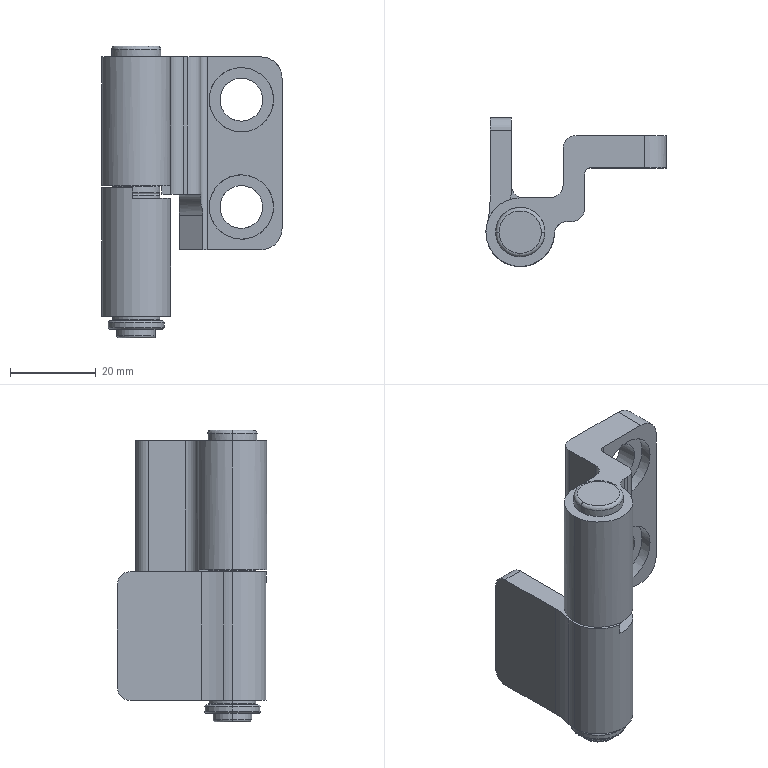Part | NX | features BREP 6 | 6 solids | 123 faces | box 42 x 34.8 x 68 mm | volume 24506 mm3 | cylinder 58 | plane 37 | torus 20 | cone 8 | commonest cylinder face diameters 6 x15 8 x10 10 x7 11 x6 16 x6 15 x4